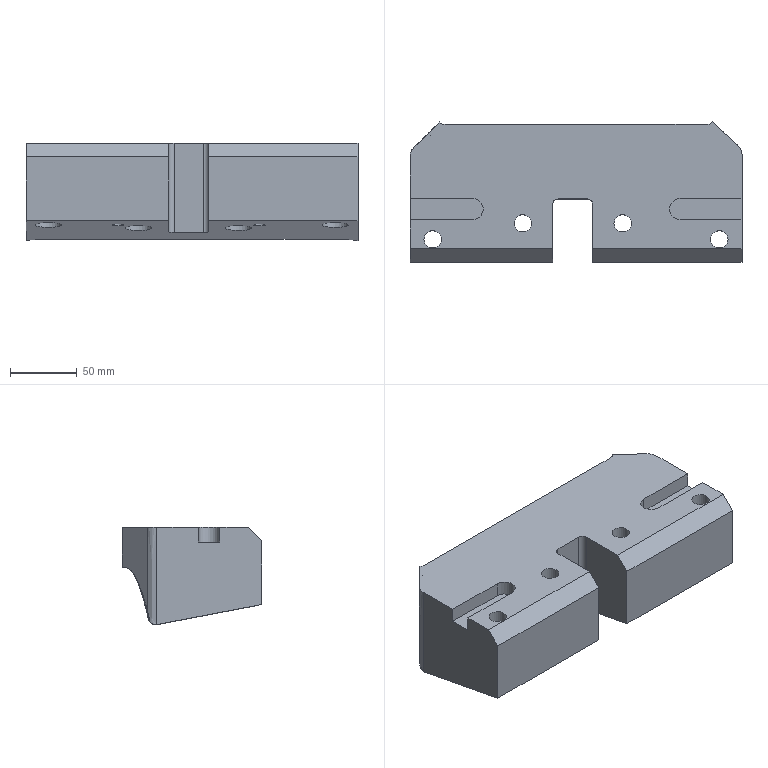Part | NX | features solid 2 | 1 solid | 70 faces | box 249.435 x 105.165 x 73.44 mm | volume 1354480 mm3 | plane 26 | spline 26 | cylinder 16 | cone 2 | commonest cylinder face diameters 13 x4 20 x4 8 x2 8.506 x2 16 x2 29 x2